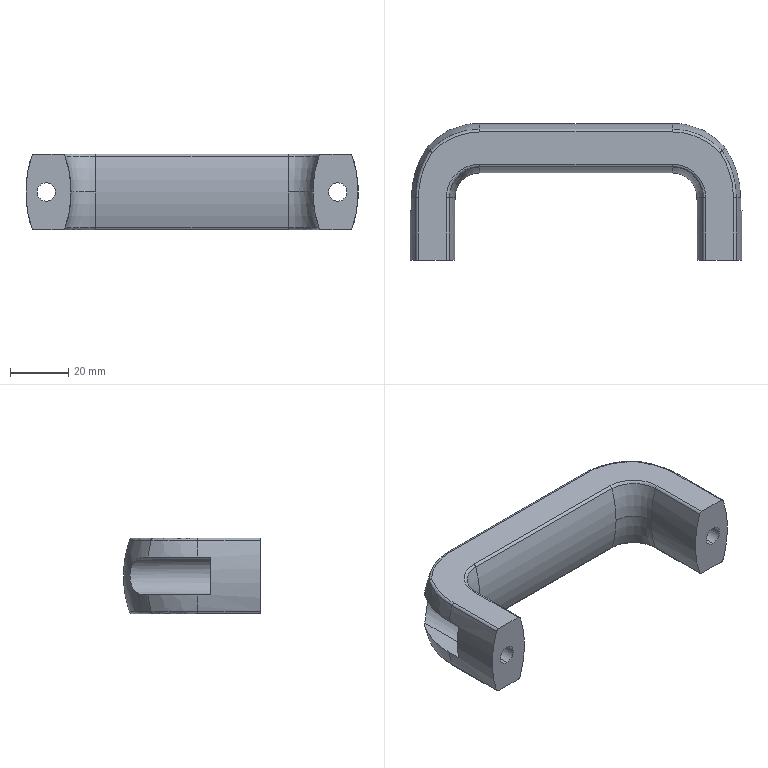Part | SolidWorks | features BaseBody 1 | 1 solid | 62 faces | box 114 x 47 x 26 mm | volume 54432 mm3 | cylinder 28 | spline 22 | plane 12 | commonest cylinder face diameters 2 x12 77 x6 6.3 x4 11 x4 13 x2